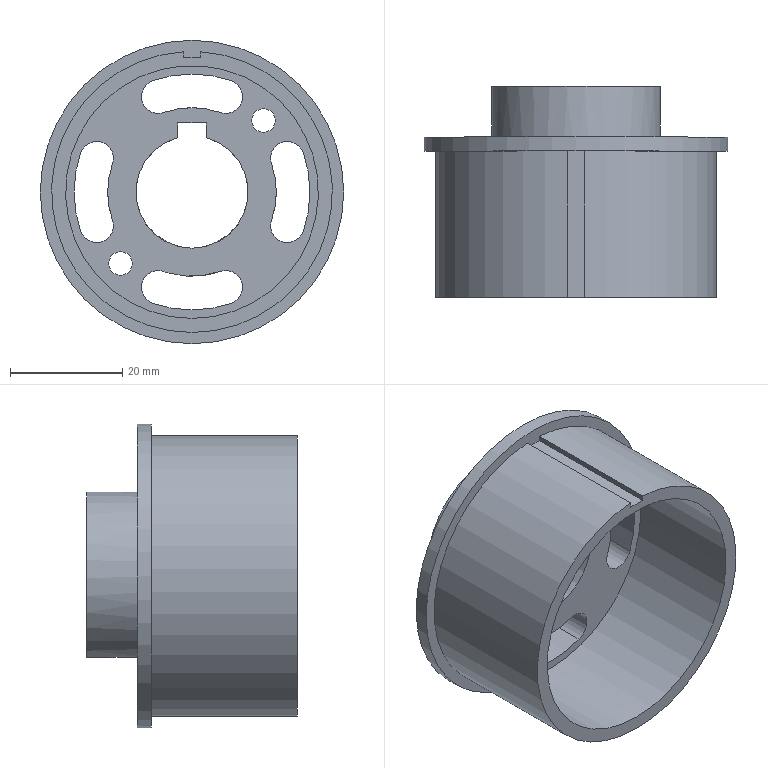Part | NX | features BREP 1 | 1 solid | 33 faces | box 54 x 37.5 x 54 mm | volume 20240 mm3 | cylinder 19 | plane 14 | commonest cylinder face diameters 6 x8 42 x4 4.2 x2 20 x1 30 x1 45 x1
STEP:
#1=CARTESIAN_POINT('',(2648.223,4020.914,39.054));
#2=VERTEX_POINT('',#1);
#3=CARTESIAN_POINT('',(2648.223,4020.914,36.954));
#4=DIRECTION('',(0.,1.,0.));
#5=DIRECTION('',(0.,0.,1.));
#6=AXIS2_PLACEMENT_3D('',#3,#4,#5);
#7=CIRCLE('',#6,2.1);
#8=EDGE_CURVE('',#2,#2,#7,.T.);
#9=ORIENTED_EDGE('',*,*,#8,.T.);
#10=EDGE_LOOP('',(#9));
#11=FACE_BOUND('',#10,.T.);
#12=CARTESIAN_POINT('',(2648.223,4013.914,39.054));
#13=VERTEX_POINT('',#12);
#14=CARTESIAN_POINT('',(2648.223,4013.914,36.954));
#15=DIRECTION('',(0.,1.,0.));
#16=DIRECTION('',(0.,0.,1.));
#17=AXIS2_PLACEMENT_3D('',#14,#15,#16);
#18=CIRCLE('',#17,2.1);
#19=EDGE_CURVE('',#13,#13,#18,.T.);
#20=ORIENTED_EDGE('',*,*,#19,.F.);
#21=EDGE_LOOP('',(#20));
#22=FACE_BOUND('',#21,.T.);
#23=CARTESIAN_POINT('',(2648.223,4020.914,36.954));
#24=DIRECTION('',(0.,1.,0.));
#25=DIRECTION('',(0.,0.,1.));
#26=AXIS2_PLACEMENT_3D('',#23,#24,#25);
#27=CYLINDRICAL_SURFACE('',#26,2.1);
#28=ADVANCED_FACE('',(#11,#22),#27,.F.);
#29=CARTESIAN_POINT('',(2673.679,4020.914,64.51));
#30=VERTEX_POINT('',#29);
#31=CARTESIAN_POINT('',(2673.679,4020.914,62.41));
#32=DIRECTION('',(0.,1.,0.));
#33=DIRECTION('',(0.,0.,1.));
#34=AXIS2_PLACEMENT_3D('',#31,#32,#33);
#35=CIRCLE('',#34,2.1);
#36=EDGE_CURVE('',#30,#30,#35,.T.);
#37=ORIENTED_EDGE('',*,*,#36,.T.);
#38=EDGE_LOOP('',(#37));
#39=FACE_BOUND('',#38,.T.);
#40=CARTESIAN_POINT('',(2673.679,4013.914,64.51));
#41=VERTEX_POINT('',#40);
#42=CARTESIAN_POINT('',(2673.679,4013.914,62.41));
#43=DIRECTION('',(0.,1.,0.));
#44=DIRECTION('',(0.,0.,1.));
#45=AXIS2_PLACEMENT_3D('',#42,#43,#44);
#46=CIRCLE('',#45,2.1);
#47=EDGE_CURVE('',#41,#41,#46,.T.);
#48=ORIENTED_EDGE('',*,*,#47,.F.);
#49=EDGE_LOOP('',(#48));
#50=FACE_BOUND('',#49,.T.);
#51=CARTESIAN_POINT('',(2673.679,4020.914,62.41));
#52=DIRECTION('',(0.,1.,0.));
#53=DIRECTION('',(0.,0.,1.));
#54=AXIS2_PLACEMENT_3D('',#51,#52,#53);
#55=CYLINDRICAL_SURFACE('',#54,2.1);
#56=ADVANCED_FACE('',(#39,#50),#55,.F.);
#57=CARTESIAN_POINT('',(2641.152,4013.914,56.682));
#58=VERTEX_POINT('',#57);
#59=CARTESIAN_POINT('',(2646.809,4013.914,54.682));
#60=VERTEX_POINT('',#59);
#61=CARTESIAN_POINT('',(2643.98,4013.914,55.682));
#62=DIRECTION('',(0.,1.,0.));
#63=DIRECTION('',(0.,0.,1.));
#64=AXIS2_PLACEMENT_3D('',#61,#62,#63);
#65=CIRCLE('',#64,3.);
#66=EDGE_CURVE('',#58,#60,#65,.T.);
#67=ORIENTED_EDGE('',*,*,#66,.F.);
#68=CARTESIAN_POINT('',(2641.152,4020.914,56.682));
#69=VERTEX_POINT('',#68);
#70=CARTESIAN_POINT('',(2641.152,4010.914,56.682));
#71=DIRECTION('',(0.,1.,0.));
#72=VECTOR('',#71,1000.);
#73=LINE('',#70,#72);
#74=EDGE_CURVE('',#58,#69,#73,.T.);
#75=ORIENTED_EDGE('',*,*,#74,.T.);
#76=CARTESIAN_POINT('',(2646.809,4020.914,54.682));
#77=VERTEX_POINT('',#76);
#78=CARTESIAN_POINT('',(2643.98,4020.914,55.682));
#79=DIRECTION('',(0.,1.,0.));
#80=DIRECTION('',(1.,0.,0.));
#81=AXIS2_PLACEMENT_3D('',#78,#79,#80);
#82=CIRCLE('',#81,3.);
#83=EDGE_CURVE('',#69,#77,#82,.T.);
#84=ORIENTED_EDGE('',*,*,#83,.T.);
#85=CARTESIAN_POINT('',(2646.809,4010.914,54.682));
#86=DIRECTION('',(0.,1.,0.));
#87=VECTOR('',#86,1000.);
#88=LINE('',#85,#87);
#89=EDGE_CURVE('',#60,#77,#88,.T.);
#90=ORIENTED_EDGE('',*,*,#89,.F.);
#91=EDGE_LOOP('',(#67,#75,#84,#90));
#92=FACE_BOUND('',#91,.T.);
#93=CARTESIAN_POINT('',(2643.98,4010.914,55.682));
#94=DIRECTION('',(0.,1.,0.));
#95=DIRECTION('',(0.,0.,1.));
#96=AXIS2_PLACEMENT_3D('',#93,#94,#95);
#97=CYLINDRICAL_SURFACE('',#96,3.);
#98=ADVANCED_FACE('',(#92),#97,.F.);
#99=CARTESIAN_POINT('',(2653.951,4013.914,69.481));
#100=VERTEX_POINT('',#99);
#101=CARTESIAN_POINT('',(2667.951,4013.914,69.481));
#102=VERTEX_POINT('',#101);
#103=CARTESIAN_POINT('',(2660.951,4013.914,49.682));
#104=DIRECTION('',(0.,1.,0.));
#105=DIRECTION('',(0.,0.,1.));
#106=AXIS2_PLACEMENT_3D('',#103,#104,#105);
#107=CIRCLE('',#106,21.);
#108=EDGE_CURVE('',#100,#102,#107,.T.);
#109=ORIENTED_EDGE('',*,*,#108,.F.);
#110=CARTESIAN_POINT('',(2653.951,4020.914,69.481));
#111=VERTEX_POINT('',#110);
#112=CARTESIAN_POINT('',(2653.951,4010.914,69.481));
#113=DIRECTION('',(0.,1.,0.));
#114=VECTOR('',#113,1000.);
#115=LINE('',#112,#114);
#116=EDGE_CURVE('',#100,#111,#115,.T.);
#117=ORIENTED_EDGE('',*,*,#116,.T.);
#118=CARTESIAN_POINT('',(2667.951,4020.914,69.481));
#119=VERTEX_POINT('',#118);
#120=CARTESIAN_POINT('',(2660.951,4020.914,49.682));
#121=DIRECTION('',(0.,1.,0.));
#122=DIRECTION('',(0.,0.,-1.));
#123=AXIS2_PLACEMENT_3D('',#120,#121,#122);
#124=CIRCLE('',#123,21.);
#125=EDGE_CURVE('',#111,#119,#124,.T.);
#126=ORIENTED_EDGE('',*,*,#125,.T.);
#127=CARTESIAN_POINT('',(2667.951,4010.914,69.481));
#128=DIRECTION('',(0.,1.,0.));
#129=VECTOR('',#128,1000.);
#130=LINE('',#127,#129);
#131=EDGE_CURVE('',#102,#119,#130,.T.);
#132=ORIENTED_EDGE('',*,*,#131,.F.);
#133=EDGE_LOOP('',(#109,#117,#126,#132));
#134=FACE_BOUND('',#133,.T.);
#135=CARTESIAN_POINT('',(2660.951,4010.914,49.682));
#136=DIRECTION('',(0.,1.,0.));
#137=DIRECTION('',(0.,0.,1.));
#138=AXIS2_PLACEMENT_3D('',#135,#136,#137);
#139=CYLINDRICAL_SURFACE('',#138,21.);
#140=ADVANCED_FACE('',(#134),#139,.F.);
#141=CARTESIAN_POINT('',(2675.093,4013.914,54.682));
#142=VERTEX_POINT('',#141);
#143=CARTESIAN_POINT('',(2680.75,4013.914,56.682));
#144=VERTEX_POINT('',#143);
#145=CARTESIAN_POINT('',(2677.922,4013.914,55.682));
#146=DIRECTION('',(0.,1.,0.));
#147=DIRECTION('',(0.,0.,1.));
#148=AXIS2_PLACEMENT_3D('',#145,#146,#147);
#149=CIRCLE('',#148,3.);
#150=EDGE_CURVE('',#142,#144,#149,.T.);
#151=ORIENTED_EDGE('',*,*,#150,.F.);
#152=CARTESIAN_POINT('',(2675.093,4020.914,54.682));
#153=VERTEX_POINT('',#152);
#154=CARTESIAN_POINT('',(2675.093,4010.914,54.682));
#155=DIRECTION('',(0.,1.,0.));
#156=VECTOR('',#155,1000.);
#157=LINE('',#154,#156);
#158=EDGE_CURVE('',#142,#153,#157,.T.);
#159=ORIENTED_EDGE('',*,*,#158,.T.);
#160=CARTESIAN_POINT('',(2680.75,4020.914,56.682));
#161=VERTEX_POINT('',#160);
#162=CARTESIAN_POINT('',(2677.922,4020.914,55.682));
#163=DIRECTION('',(0.,1.,0.));
#164=DIRECTION('',(-1.,0.,0.));
#165=AXIS2_PLACEMENT_3D('',#162,#163,#164);
#166=CIRCLE('',#165,3.);
#167=EDGE_CURVE('',#153,#161,#166,.T.);
#168=ORIENTED_EDGE('',*,*,#167,.T.);
#169=CARTESIAN_POINT('',(2680.75,4010.914,56.682));
#170=DIRECTION('',(0.,1.,0.));
#171=VECTOR('',#170,1000.);
#172=LINE('',#169,#171);
#173=EDGE_CURVE('',#144,#161,#172,.T.);
#174=ORIENTED_EDGE('',*,*,#173,.F.);
#175=EDGE_LOOP('',(#151,#159,#168,#174));
#176=FACE_BOUND('',#175,.T.);
#177=CARTESIAN_POINT('',(2677.922,4010.914,55.682));
#178=DIRECTION('',(0.,1.,0.));
#179=DIRECTION('',(0.,0.,1.));
#180=AXIS2_PLACEMENT_3D('',#177,#178,#179);
#181=CYLINDRICAL_SURFACE('',#180,3.);
#182=ADVANCED_FACE('',(#176),#181,.F.);
#183=CARTESIAN_POINT('',(2653.951,4013.914,29.883));
#184=VERTEX_POINT('',#183);
#185=CARTESIAN_POINT('',(2655.951,4013.914,35.54));
#186=VERTEX_POINT('',#185);
#187=CARTESIAN_POINT('',(2654.951,4013.914,32.712));
#188=DIRECTION('',(0.,1.,0.));
#189=DIRECTION('',(0.,0.,1.));
#190=AXIS2_PLACEMENT_3D('',#187,#188,#189);
#191=CIRCLE('',#190,3.);
#192=EDGE_CURVE('',#184,#186,#191,.T.);
#193=ORIENTED_EDGE('',*,*,#192,.F.);
#194=CARTESIAN_POINT('',(2653.951,4020.914,29.883));
#195=VERTEX_POINT('',#194);
#196=CARTESIAN_POINT('',(2653.951,4010.914,29.883));
#197=DIRECTION('',(0.,1.,0.));
#198=VECTOR('',#197,1000.);
#199=LINE('',#196,#198);
#200=EDGE_CURVE('',#184,#195,#199,.T.);
#201=ORIENTED_EDGE('',*,*,#200,.T.);
#202=CARTESIAN_POINT('',(2655.951,4020.914,35.54));
#203=VERTEX_POINT('',#202);
#204=CARTESIAN_POINT('',(2654.951,4020.914,32.712));
#205=DIRECTION('',(0.,1.,0.));
#206=DIRECTION('',(0.,0.,1.));
#207=AXIS2_PLACEMENT_3D('',#204,#205,#206);
#208=CIRCLE('',#207,3.);
#209=EDGE_CURVE('',#195,#203,#208,.T.);
#210=ORIENTED_EDGE('',*,*,#209,.T.);
#211=CARTESIAN_POINT('',(2655.951,4010.914,35.54));
#212=DIRECTION('',(0.,1.,0.));
#213=VECTOR('',#212,1000.);
#214=LINE('',#211,#213);
#215=EDGE_CURVE('',#186,#203,#214,.T.);
#216=ORIENTED_EDGE('',*,*,#215,.F.);
#217=EDGE_LOOP('',(#193,#201,#210,#216));
#218=FACE_BOUND('',#217,.T.);
#219=CARTESIAN_POINT('',(2654.951,4010.914,32.712));
#220=DIRECTION('',(0.,1.,0.));
#221=DIRECTION('',(0.,0.,1.));
#222=AXIS2_PLACEMENT_3D('',#219,#220,#221);
#223=CYLINDRICAL_SURFACE('',#222,3.);
#224=ADVANCED_FACE('',(#218),#223,.F.);
#225=CARTESIAN_POINT('',(2665.951,4013.914,35.54));
#226=VERTEX_POINT('',#225);
#227=CARTESIAN_POINT('',(2667.951,4013.914,29.883));
#228=VERTEX_POINT('',#227);
#229=CARTESIAN_POINT('',(2666.951,4013.914,32.712));
#230=DIRECTION('',(0.,1.,0.));
#231=DIRECTION('',(0.,0.,1.));
#232=AXIS2_PLACEMENT_3D('',#229,#230,#231);
#233=CIRCLE('',#232,3.);
#234=EDGE_CURVE('',#226,#228,#233,.T.);
#235=ORIENTED_EDGE('',*,*,#234,.F.);
#236=CARTESIAN_POINT('',(2665.951,4020.914,35.54));
#237=VERTEX_POINT('',#236);
#238=CARTESIAN_POINT('',(2665.951,4010.914,35.54));
#239=DIRECTION('',(0.,1.,0.));
#240=VECTOR('',#239,1000.);
#241=LINE('',#238,#240);
#242=EDGE_CURVE('',#226,#237,#241,.T.);
#243=ORIENTED_EDGE('',*,*,#242,.T.);
#244=CARTESIAN_POINT('',(2667.951,4020.914,29.883));
#245=VERTEX_POINT('',#244);
#246=CARTESIAN_POINT('',(2666.951,4020.914,32.712));
#247=DIRECTION('',(0.,1.,0.));
#248=DIRECTION('',(0.,0.,1.));
#249=AXIS2_PLACEMENT_3D('',#246,#247,#248);
#250=CIRCLE('',#249,3.);
#251=EDGE_CURVE('',#237,#245,#250,.T.);
#252=ORIENTED_EDGE('',*,*,#251,.T.);
#253=CARTESIAN_POINT('',(2667.951,4010.914,29.883));
#254=DIRECTION('',(0.,1.,0.));
#255=VECTOR('',#254,1000.);
#256=LINE('',#253,#255);
#257=EDGE_CURVE('',#228,#245,#256,.T.);
#258=ORIENTED_EDGE('',*,*,#257,.F.);
#259=EDGE_LOOP('',(#235,#243,#252,#258));
#260=FACE_BOUND('',#259,.T.);
#261=CARTESIAN_POINT('',(2666.951,4010.914,32.712));
#262=DIRECTION('',(0.,1.,0.));
#263=DIRECTION('',(0.,0.,1.));
#264=AXIS2_PLACEMENT_3D('',#261,#262,#263);
#265=CYLINDRICAL_SURFACE('',#264,3.);
#266=ADVANCED_FACE('',(#260),#265,.F.);
#267=CARTESIAN_POINT('',(2660.951,3992.414,27.182));
#268=VERTEX_POINT('',#267);
#269=CARTESIAN_POINT('',(2660.951,3992.414,49.682));
#270=DIRECTION('',(0.,-1.,0.));
#271=DIRECTION('',(0.,0.,-1.));
#272=AXIS2_PLACEMENT_3D('',#269,#270,#271);
#273=CIRCLE('',#272,22.5);
#274=EDGE_CURVE('',#268,#268,#273,.T.);
#275=ORIENTED_EDGE('',*,*,#274,.T.);
#276=EDGE_LOOP('',(#275));
#277=FACE_BOUND('',#276,.T.);
#278=CARTESIAN_POINT('',(2660.951,4013.914,27.182));
#279=VERTEX_POINT('',#278);
#280=CARTESIAN_POINT('',(2660.951,4013.914,49.682));
#281=DIRECTION('',(0.,-1.,0.));
#282=DIRECTION('',(0.,0.,-1.));
#283=AXIS2_PLACEMENT_3D('',#280,#281,#282);
#284=CIRCLE('',#283,22.5);
#285=EDGE_CURVE('',#279,#279,#284,.T.);
#286=ORIENTED_EDGE('',*,*,#285,.F.);
#287=EDGE_LOOP('',(#286));
#288=FACE_BOUND('',#287,.T.);
#289=CARTESIAN_POINT('',(2660.951,4029.914,49.682));
#290=DIRECTION('',(0.,-1.,0.));
#291=DIRECTION('',(0.,0.,-1.));
#292=AXIS2_PLACEMENT_3D('',#289,#290,#291);
#293=CYLINDRICAL_SURFACE('',#292,22.5);
#294=ADVANCED_FACE('',(#277,#288),#293,.F.);
#295=CARTESIAN_POINT('',(2660.951,4013.914,49.682));
#296=DIRECTION('',(0.,-1.,0.));
#297=DIRECTION('',(0.,0.,1.));
#298=AXIS2_PLACEMENT_3D('',#295,#296,#297);
#299=CIRCLE('',#298,15.);
#300=EDGE_CURVE('',#186,#226,#299,.T.);
#301=ORIENTED_EDGE('',*,*,#300,.F.);
#302=ORIENTED_EDGE('',*,*,#215,.T.);
#303=CARTESIAN_POINT('',(2646.809,4020.914,44.682));
#304=VERTEX_POINT('',#303);
#305=CARTESIAN_POINT('',(2660.951,4020.914,49.682));
#306=DIRECTION('',(0.,1.,0.));
#307=DIRECTION('',(0.,0.,1.));
#308=AXIS2_PLACEMENT_3D('',#305,#306,#307);
#309=CIRCLE('',#308,15.);
#310=EDGE_CURVE('',#203,#304,#309,.T.);
#311=ORIENTED_EDGE('',*,*,#310,.T.);
#312=CARTESIAN_POINT('',(2646.809,4013.914,44.682));
#313=VERTEX_POINT('',#312);
#314=CARTESIAN_POINT('',(2646.809,4010.914,44.682));
#315=DIRECTION('',(0.,1.,0.));
#316=VECTOR('',#315,1000.);
#317=LINE('',#314,#316);
#318=EDGE_CURVE('',#313,#304,#317,.T.);
#319=ORIENTED_EDGE('',*,*,#318,.F.);
#320=CARTESIAN_POINT('',(2660.951,4013.914,49.682));
#321=DIRECTION('',(0.,-1.,0.));
#322=DIRECTION('',(0.,0.,1.));
#323=AXIS2_PLACEMENT_3D('',#320,#321,#322);
#324=CIRCLE('',#323,15.);
#325=EDGE_CURVE('',#60,#313,#324,.T.);
#326=ORIENTED_EDGE('',*,*,#325,.F.);
#327=ORIENTED_EDGE('',*,*,#89,.T.);
#328=CARTESIAN_POINT('',(2655.951,4020.914,63.825));
#329=VERTEX_POINT('',#328);
#330=CARTESIAN_POINT('',(2660.951,4020.914,49.682));
#331=DIRECTION('',(0.,1.,0.));
#332=DIRECTION('',(0.,0.,1.));
#333=AXIS2_PLACEMENT_3D('',#330,#331,#332);
#334=CIRCLE('',#333,15.);
#335=EDGE_CURVE('',#77,#329,#334,.T.);
#336=ORIENTED_EDGE('',*,*,#335,.T.);
#337=CARTESIAN_POINT('',(2655.951,4013.914,63.825));
#338=VERTEX_POINT('',#337);
#339=CARTESIAN_POINT('',(2655.951,4010.914,63.825));
#340=DIRECTION('',(0.,1.,0.));
#341=VECTOR('',#340,1000.);
#342=LINE('',#339,#341);
#343=EDGE_CURVE('',#338,#329,#342,.T.);
#344=ORIENTED_EDGE('',*,*,#343,.F.);
#345=CARTESIAN_POINT('',(2665.951,4013.914,63.825));
#346=VERTEX_POINT('',#345);
#347=CARTESIAN_POINT('',(2660.951,4013.914,49.682));
#348=DIRECTION('',(0.,-1.,0.));
#349=DIRECTION('',(0.,0.,1.));
#350=AXIS2_PLACEMENT_3D('',#347,#348,#349);
#351=CIRCLE('',#350,15.);
#352=EDGE_CURVE('',#346,#338,#351,.T.);
#353=ORIENTED_EDGE('',*,*,#352,.F.);
#354=CARTESIAN_POINT('',(2665.951,4020.914,63.825));
#355=VERTEX_POINT('',#354);
#356=CARTESIAN_POINT('',(2665.951,4010.914,63.825));
#357=DIRECTION('',(0.,1.,0.));
#358=VECTOR('',#357,1000.);
#359=LINE('',#356,#358);
#360=EDGE_CURVE('',#346,#355,#359,.T.);
#361=ORIENTED_EDGE('',*,*,#360,.T.);
#362=CARTESIAN_POINT('',(2660.951,4020.914,49.682));
#363=DIRECTION('',(0.,1.,0.));
#364=DIRECTION('',(0.,0.,1.));
#365=AXIS2_PLACEMENT_3D('',#362,#363,#364);
#366=CIRCLE('',#365,15.);
#367=EDGE_CURVE('',#355,#153,#366,.T.);
#368=ORIENTED_EDGE('',*,*,#367,.T.);
#369=ORIENTED_EDGE('',*,*,#158,.F.);
#370=CARTESIAN_POINT('',(2675.093,4013.914,44.682));
#371=VERTEX_POINT('',#370);
#372=CARTESIAN_POINT('',(2660.951,4013.914,49.682));
#373=DIRECTION('',(0.,-1.,0.));
#374=DIRECTION('',(0.,0.,1.));
#375=AXIS2_PLACEMENT_3D('',#372,#373,#374);
#376=CIRCLE('',#375,15.);
#377=EDGE_CURVE('',#371,#142,#376,.T.);
#378=ORIENTED_EDGE('',*,*,#377,.F.);
#379=CARTESIAN_POINT('',(2675.093,4020.914,44.682));
#380=VERTEX_POINT('',#379);
#381=CARTESIAN_POINT('',(2675.093,4010.914,44.682));
#382=DIRECTION('',(0.,1.,0.));
#383=VECTOR('',#382,1000.);
#384=LINE('',#381,#383);
#385=EDGE_CURVE('',#371,#380,#384,.T.);
#386=ORIENTED_EDGE('',*,*,#385,.T.);
#387=CARTESIAN_POINT('',(2660.951,4020.914,49.682));
#388=DIRECTION('',(0.,1.,0.));
#389=DIRECTION('',(0.,0.,1.));
#390=AXIS2_PLACEMENT_3D('',#387,#388,#389);
#391=CIRCLE('',#390,15.);
#392=EDGE_CURVE('',#380,#237,#391,.T.);
#393=ORIENTED_EDGE('',*,*,#392,.T.);
#394=ORIENTED_EDGE('',*,*,#242,.F.);
#395=EDGE_LOOP('',(#301,#302,#311,#319,#326,#327,#336,#344,#353,#361,#368,#369,#378,#386,#393,#394));
#396=FACE_BOUND('',#395,.T.);
#397=CARTESIAN_POINT('',(2656.951,4029.914,35.226));
#398=VERTEX_POINT('',#397);
#399=CARTESIAN_POINT('',(2664.951,4029.914,35.226));
#400=VERTEX_POINT('',#399);
#401=CARTESIAN_POINT('',(2660.951,4029.914,49.682));
#402=DIRECTION('',(0.,1.,0.));
#403=DIRECTION('',(0.,0.,1.));
#404=AXIS2_PLACEMENT_3D('',#401,#402,#403);
#405=CIRCLE('',#404,15.);
#406=EDGE_CURVE('',#398,#400,#405,.T.);
#407=ORIENTED_EDGE('',*,*,#406,.F.);
#408=CARTESIAN_POINT('',(2656.951,4020.914,35.226));
#409=VERTEX_POINT('',#408);
#410=CARTESIAN_POINT('',(2656.951,4020.914,35.226));
#411=DIRECTION('',(0.,1.,0.));
#412=VECTOR('',#411,1000.);
#413=LINE('',#410,#412);
#414=EDGE_CURVE('',#409,#398,#413,.T.);
#415=ORIENTED_EDGE('',*,*,#414,.F.);
#416=CARTESIAN_POINT('',(2664.951,4020.914,35.226));
#417=VERTEX_POINT('',#416);
#418=CARTESIAN_POINT('',(2660.951,4020.914,49.682));
#419=DIRECTION('',(0.,-1.,0.));
#420=DIRECTION('',(0.,0.,1.));
#421=AXIS2_PLACEMENT_3D('',#418,#419,#420);
#422=CIRCLE('',#421,15.);
#423=EDGE_CURVE('',#409,#417,#422,.T.);
#424=ORIENTED_EDGE('',*,*,#423,.T.);
#425=CARTESIAN_POINT('',(2664.951,4020.914,35.226));
#426=DIRECTION('',(0.,1.,0.));
#427=VECTOR('',#426,1000.);
#428=LINE('',#425,#427);
#429=EDGE_CURVE('',#417,#400,#428,.T.);
#430=ORIENTED_EDGE('',*,*,#429,.T.);
#431=EDGE_LOOP('',(#407,#415,#424,#430));
#432=FACE_BOUND('',#431,.T.);
#433=CARTESIAN_POINT('',(2660.951,4029.914,49.682));
#434=DIRECTION('',(0.,-1.,0.));
#435=DIRECTION('',(0.,0.,-1.));
#436=AXIS2_PLACEMENT_3D('',#433,#434,#435);
#437=CYLINDRICAL_SURFACE('',#436,15.);
#438=ADVANCED_FACE('',(#396,#432),#437,.T.);
#439=CARTESIAN_POINT('',(2660.951,4018.414,22.682));
#440=VERTEX_POINT('',#439);
#441=CARTESIAN_POINT('',(2660.951,4018.414,49.682));
#442=DIRECTION('',(0.,-1.,0.));
#443=DIRECTION('',(0.,0.,-1.));
#444=AXIS2_PLACEMENT_3D('',#441,#442,#443);
#445=CIRCLE('',#444,27.);
#446=EDGE_CURVE('',#440,#440,#445,.T.);
#447=ORIENTED_EDGE('',*,*,#446,.F.);
#448=EDGE_LOOP('',(#447));
#449=FACE_BOUND('',#448,.T.);
#450=CARTESIAN_POINT('',(2660.951,4020.914,22.682));
#451=VERTEX_POINT('',#450);
#452=CARTESIAN_POINT('',(2660.951,4020.914,49.682));
#453=DIRECTION('',(0.,-1.,0.));
#454=DIRECTION('',(0.,0.,-1.));
#455=AXIS2_PLACEMENT_3D('',#452,#453,#454);
#456=CIRCLE('',#455,27.);
#457=EDGE_CURVE('',#451,#451,#456,.T.);
#458=ORIENTED_EDGE('',*,*,#457,.T.);
#459=EDGE_LOOP('',(#458));
#460=FACE_BOUND('',#459,.T.);
#461=CARTESIAN_POINT('',(2660.951,4020.914,49.682));
#462=DIRECTION('',(0.,-1.,0.));
#463=DIRECTION('',(0.,0.,-1.));
#464=AXIS2_PLACEMENT_3D('',#461,#462,#463);
#465=CYLINDRICAL_SURFACE('',#464,27.);
#466=ADVANCED_FACE('',(#449,#460),#465,.T.);
#467=CARTESIAN_POINT('',(2656.951,4020.914,40.517));
#468=VERTEX_POINT('',#467);
#469=CARTESIAN_POINT('',(2664.951,4020.914,40.517));
#470=VERTEX_POINT('',#469);
#471=CARTESIAN_POINT('',(2660.951,4020.914,49.682));
#472=DIRECTION('',(0.,-1.,0.));
#473=DIRECTION('',(0.,0.,-1.));
#474=AXIS2_PLACEMENT_3D('',#471,#472,#473);
#475=CIRCLE('',#474,10.);
#476=EDGE_CURVE('',#468,#470,#475,.T.);
#477=ORIENTED_EDGE('',*,*,#476,.F.);
#478=CARTESIAN_POINT('',(2656.951,4029.914,40.517));
#479=VERTEX_POINT('',#478);
#480=CARTESIAN_POINT('',(2656.951,4020.914,40.517));
#481=DIRECTION('',(0.,1.,0.));
#482=VECTOR('',#481,1000.);
#483=LINE('',#480,#482);
#484=EDGE_CURVE('',#468,#479,#483,.T.);
#485=ORIENTED_EDGE('',*,*,#484,.T.);
#486=CARTESIAN_POINT('',(2658.451,4029.914,59.365));
#487=VERTEX_POINT('',#486);
#488=CARTESIAN_POINT('',(2660.951,4029.914,49.682));
#489=DIRECTION('',(0.,-1.,0.));
#490=DIRECTION('',(0.,0.,-1.));
#491=AXIS2_PLACEMENT_3D('',#488,#489,#490);
#492=CIRCLE('',#491,10.);
#493=EDGE_CURVE('',#487,#479,#492,.T.);
#494=ORIENTED_EDGE('',*,*,#493,.F.);
#495=CARTESIAN_POINT('',(2658.451,4013.914,59.365));
#496=VERTEX_POINT('',#495);
#497=CARTESIAN_POINT('',(2658.451,4029.914,59.365));
#498=DIRECTION('',(0.,1.,0.));
#499=VECTOR('',#498,1000.);
#500=LINE('',#497,#499);
#501=EDGE_CURVE('',#496,#487,#500,.T.);
#502=ORIENTED_EDGE('',*,*,#501,.F.);
#503=CARTESIAN_POINT('',(2663.451,4013.914,59.365));
#504=VERTEX_POINT('',#503);
#505=CARTESIAN_POINT('',(2660.951,4013.914,49.682));
#506=DIRECTION('',(0.,-1.,0.));
#507=DIRECTION('',(0.,0.,-1.));
#508=AXIS2_PLACEMENT_3D('',#505,#506,#507);
#509=CIRCLE('',#508,10.);
#510=EDGE_CURVE('',#496,#504,#509,.T.);
#511=ORIENTED_EDGE('',*,*,#510,.T.);
#512=CARTESIAN_POINT('',(2663.451,4029.914,59.365));
#513=VERTEX_POINT('',#512);
#514=CARTESIAN_POINT('',(2663.451,4029.914,59.365));
#515=DIRECTION('',(0.,-1.,0.));
#516=VECTOR('',#515,1000.);
#517=LINE('',#514,#516);
#518=EDGE_CURVE('',#513,#504,#517,.T.);
#519=ORIENTED_EDGE('',*,*,#518,.F.);
#520=CARTESIAN_POINT('',(2664.951,4029.914,40.517));
#521=VERTEX_POINT('',#520);
#522=CARTESIAN_POINT('',(2660.951,4029.914,49.682));
#523=DIRECTION('',(0.,-1.,0.));
#524=DIRECTION('',(0.,0.,-1.));
#525=AXIS2_PLACEMENT_3D('',#522,#523,#524);
#526=CIRCLE('',#525,10.);
#527=EDGE_CURVE('',#521,#513,#526,.T.);
#528=ORIENTED_EDGE('',*,*,#527,.F.);
#529=CARTESIAN_POINT('',(2664.951,4020.914,40.517));
#530=DIRECTION('',(0.,1.,0.));
#531=VECTOR('',#530,1000.);
#532=LINE('',#529,#531);
#533=EDGE_CURVE('',#470,#521,#532,.T.);
#534=ORIENTED_EDGE('',*,*,#533,.F.);
#535=EDGE_LOOP('',(#477,#485,#494,#502,#511,#519,#528,#534));
#536=FACE_BOUND('',#535,.T.);
#537=CARTESIAN_POINT('',(2660.951,4029.914,49.682));
#538=DIRECTION('',(0.,-1.,0.));
#539=DIRECTION('',(0.,0.,-1.));
#540=AXIS2_PLACEMENT_3D('',#537,#538,#539);
#541=CYLINDRICAL_SURFACE('',#540,10.);
#542=ADVANCED_FACE('',(#536),#541,.F.);
#543=ORIENTED_EDGE('',*,*,#423,.F.);
#544=CARTESIAN_POINT('',(2656.951,4020.914,35.226));
#545=DIRECTION('',(0.,0.,1.));
#546=VECTOR('',#545,1000.);
#547=LINE('',#544,#546);
#548=EDGE_CURVE('',#409,#468,#547,.T.);
#549=ORIENTED_EDGE('',*,*,#548,.T.);
#550=ORIENTED_EDGE('',*,*,#476,.T.);
#551=CARTESIAN_POINT('',(2664.951,4020.914,40.517));
#552=DIRECTION('',(0.,0.,-1.));
#553=VECTOR('',#552,1000.);
#554=LINE('',#551,#553);
#555=EDGE_CURVE('',#470,#417,#554,.T.);
#556=ORIENTED_EDGE('',*,*,#555,.T.);
#557=EDGE_LOOP('',(#543,#549,#550,#556));
#558=FACE_BOUND('',#557,.T.);
#559=CARTESIAN_POINT('',(2687.951,4020.914,49.682));
#560=DIRECTION('',(0.,1.,0.));
#561=DIRECTION('',(0.,0.,1.));
#562=AXIS2_PLACEMENT_3D('',#559,#560,#561);
#563=PLANE('',#562);
#564=ADVANCED_FACE('',(#558),#563,.T.);
#565=CARTESIAN_POINT('',(2658.451,4029.914,61.982));
#566=VERTEX_POINT('',#565);
#567=CARTESIAN_POINT('',(2663.451,4029.914,61.982));
#568=VERTEX_POINT('',#567);
#569=CARTESIAN_POINT('',(2663.451,4029.914,61.982));
#570=DIRECTION('',(1.,0.,0.));
#571=VECTOR('',#570,1000.);
#572=LINE('',#569,#571);
#573=EDGE_CURVE('',#566,#568,#572,.T.);
#574=ORIENTED_EDGE('',*,*,#573,.F.);
#575=CARTESIAN_POINT('',(2658.451,4029.914,57.682));
#576=DIRECTION('',(0.,0.,1.));
#577=VECTOR('',#576,1000.);
#578=LINE('',#575,#577);
#579=EDGE_CURVE('',#487,#566,#578,.T.);
#580=ORIENTED_EDGE('',*,*,#579,.F.);
#581=ORIENTED_EDGE('',*,*,#493,.T.);
#582=CARTESIAN_POINT('',(2656.951,4029.914,35.226));
#583=DIRECTION('',(0.,0.,1.));
#584=VECTOR('',#583,1000.);
#585=LINE('',#582,#584);
#586=EDGE_CURVE('',#398,#479,#585,.T.);
#587=ORIENTED_EDGE('',*,*,#586,.F.);
#588=ORIENTED_EDGE('',*,*,#406,.T.);
#589=CARTESIAN_POINT('',(2664.951,4029.914,40.517));
#590=DIRECTION('',(0.,0.,-1.));
#591=VECTOR('',#590,1000.);
#592=LINE('',#589,#591);
#593=EDGE_CURVE('',#521,#400,#592,.T.);
#594=ORIENTED_EDGE('',*,*,#593,.F.);
#595=ORIENTED_EDGE('',*,*,#527,.T.);
#596=CARTESIAN_POINT('',(2663.451,4029.914,57.682));
#597=DIRECTION('',(0.,0.,1.));
#598=VECTOR('',#597,1000.);
#599=LINE('',#596,#598);
#600=EDGE_CURVE('',#513,#568,#599,.T.);
#601=ORIENTED_EDGE('',*,*,#600,.T.);
#602=EDGE_LOOP('',(#574,#580,#581,#587,#588,#594,#595,#601));
#603=FACE_BOUND('',#602,.T.);
#604=CARTESIAN_POINT('',(2660.951,4029.914,49.682));
#605=DIRECTION('',(0.,1.,0.));
#606=DIRECTION('',(0.,0.,1.));
#607=AXIS2_PLACEMENT_3D('',#604,#605,#606);
#608=PLANE('',#607);
#609=ADVANCED_FACE('',(#603),#608,.T.);
#610=ORIENTED_EDGE('',*,*,#19,.T.);
#611=EDGE_LOOP('',(#610));
#612=FACE_BOUND('',#611,.T.);
#613=ORIENTED_EDGE('',*,*,#47,.T.);
#614=EDGE_LOOP('',(#613));
#615=FACE_BOUND('',#614,.T.);
#616=ORIENTED_EDGE('',*,*,#325,.T.);
#617=CARTESIAN_POINT('',(2641.152,4013.914,42.682));
#618=VERTEX_POINT('',#617);
#619=CARTESIAN_POINT('',(2643.98,4013.914,43.682));
#620=DIRECTION('',(0.,1.,0.));
#621=DIRECTION('',(0.,0.,1.));
#622=AXIS2_PLACEMENT_3D('',#619,#620,#621);
#623=CIRCLE('',#622,3.);
#624=EDGE_CURVE('',#313,#618,#623,.T.);
#625=ORIENTED_EDGE('',*,*,#624,.T.);
#626=CARTESIAN_POINT('',(2660.951,4013.914,49.682));
#627=DIRECTION('',(0.,1.,0.));
#628=DIRECTION('',(0.,0.,1.));
#629=AXIS2_PLACEMENT_3D('',#626,#627,#628);
#630=CIRCLE('',#629,21.);
#631=EDGE_CURVE('',#618,#58,#630,.T.);
#632=ORIENTED_EDGE('',*,*,#631,.T.);
#633=ORIENTED_EDGE('',*,*,#66,.T.);
#634=EDGE_LOOP('',(#616,#625,#632,#633));
#635=FACE_BOUND('',#634,.T.);
#636=ORIENTED_EDGE('',*,*,#352,.T.);
#637=CARTESIAN_POINT('',(2654.951,4013.914,66.653));
#638=DIRECTION('',(0.,1.,0.));
#639=DIRECTION('',(0.,0.,1.));
#640=AXIS2_PLACEMENT_3D('',#637,#638,#639);
#641=CIRCLE('',#640,3.);
#642=EDGE_CURVE('',#338,#100,#641,.T.);
#643=ORIENTED_EDGE('',*,*,#642,.T.);
#644=ORIENTED_EDGE('',*,*,#108,.T.);
#645=CARTESIAN_POINT('',(2666.951,4013.914,66.653));
#646=DIRECTION('',(0.,1.,0.));
#647=DIRECTION('',(0.,0.,1.));
#648=AXIS2_PLACEMENT_3D('',#645,#646,#647);
#649=CIRCLE('',#648,3.);
#650=EDGE_CURVE('',#102,#346,#649,.T.);
#651=ORIENTED_EDGE('',*,*,#650,.T.);
#652=EDGE_LOOP('',(#636,#643,#644,#651));
#653=FACE_BOUND('',#652,.T.);
#654=ORIENTED_EDGE('',*,*,#377,.T.);
#655=ORIENTED_EDGE('',*,*,#150,.T.);
#656=CARTESIAN_POINT('',(2680.75,4013.914,42.682));
#657=VERTEX_POINT('',#656);
#658=CARTESIAN_POINT('',(2660.951,4013.914,49.682));
#659=DIRECTION('',(0.,1.,0.));
#660=DIRECTION('',(0.,0.,1.));
#661=AXIS2_PLACEMENT_3D('',#658,#659,#660);
#662=CIRCLE('',#661,21.);
#663=EDGE_CURVE('',#144,#657,#662,.T.);
#664=ORIENTED_EDGE('',*,*,#663,.T.);
#665=CARTESIAN_POINT('',(2677.922,4013.914,43.682));
#666=DIRECTION('',(0.,1.,0.));
#667=DIRECTION('',(0.,0.,1.));
#668=AXIS2_PLACEMENT_3D('',#665,#666,#667);
#669=CIRCLE('',#668,3.);
#670=EDGE_CURVE('',#657,#371,#669,.T.);
#671=ORIENTED_EDGE('',*,*,#670,.T.);
#672=EDGE_LOOP('',(#654,#655,#664,#671));
#673=FACE_BOUND('',#672,.T.);
#674=ORIENTED_EDGE('',*,*,#192,.T.);
#675=ORIENTED_EDGE('',*,*,#300,.T.);
#676=ORIENTED_EDGE('',*,*,#234,.T.);
#677=CARTESIAN_POINT('',(2660.951,4013.914,49.682));
#678=DIRECTION('',(0.,1.,0.));
#679=DIRECTION('',(0.,0.,1.));
#680=AXIS2_PLACEMENT_3D('',#677,#678,#679);
#681=CIRCLE('',#680,21.);
#682=EDGE_CURVE('',#228,#184,#681,.T.);
#683=ORIENTED_EDGE('',*,*,#682,.T.);
#684=EDGE_LOOP('',(#674,#675,#676,#683));
#685=FACE_BOUND('',#684,.T.);
#686=ORIENTED_EDGE('',*,*,#285,.T.);
#687=EDGE_LOOP('',(#686));
#688=FACE_BOUND('',#687,.T.);
#689=CARTESIAN_POINT('',(2658.451,4013.914,61.982));
#690=VERTEX_POINT('',#689);
#691=CARTESIAN_POINT('',(2658.451,4013.914,49.682));
#692=DIRECTION('',(0.,0.,-1.));
#693=VECTOR('',#692,1000.);
#694=LINE('',#691,#693);
#695=EDGE_CURVE('',#690,#496,#694,.T.);
#696=ORIENTED_EDGE('',*,*,#695,.F.);
#697=CARTESIAN_POINT('',(2663.451,4013.914,61.982));
#698=VERTEX_POINT('',#697);
#699=CARTESIAN_POINT('',(2683.451,4013.914,61.982));
#700=DIRECTION('',(-1.,0.,0.));
#701=VECTOR('',#700,1000.);
#702=LINE('',#699,#701);
#703=EDGE_CURVE('',#698,#690,#702,.T.);
#704=ORIENTED_EDGE('',*,*,#703,.F.);
#705=CARTESIAN_POINT('',(2663.451,4013.914,49.682));
#706=DIRECTION('',(0.,0.,1.));
#707=VECTOR('',#706,1000.);
#708=LINE('',#705,#707);
#709=EDGE_CURVE('',#504,#698,#708,.T.);
#710=ORIENTED_EDGE('',*,*,#709,.F.);
#711=ORIENTED_EDGE('',*,*,#510,.F.);
#712=EDGE_LOOP('',(#696,#704,#710,#711));
#713=FACE_BOUND('',#712,.T.);
#714=CARTESIAN_POINT('',(2683.451,4013.914,49.682));
#715=DIRECTION('',(0.,1.,0.));
#716=DIRECTION('',(0.,0.,1.));
#717=AXIS2_PLACEMENT_3D('',#714,#715,#716);
#718=PLANE('',#717);
#719=ADVANCED_FACE('',(#612,#615,#635,#653,#673,#685,#688,#713),#718,.F.);
#720=ORIENTED_EDGE('',*,*,#446,.T.);
#721=EDGE_LOOP('',(#720));
#722=FACE_BOUND('',#721,.T.);
#723=CARTESIAN_POINT('',(2662.451,4018.414,74.637));
#724=VERTEX_POINT('',#723);
#725=CARTESIAN_POINT('',(2662.451,4018.414,73.682));
#726=VERTEX_POINT('',#725);
#727=CARTESIAN_POINT('',(2662.451,4018.414,73.682));
#728=DIRECTION('',(0.,0.,-1.));
#729=VECTOR('',#728,1000.);
#730=LINE('',#727,#729);
#731=EDGE_CURVE('',#724,#726,#730,.T.);
#732=ORIENTED_EDGE('',*,*,#731,.F.);
#733=CARTESIAN_POINT('',(2659.451,4018.414,74.637));
#734=VERTEX_POINT('',#733);
#735=CARTESIAN_POINT('',(2660.951,4018.414,49.682));
#736=DIRECTION('',(0.,-1.,0.));
#737=DIRECTION('',(0.,0.,-1.));
#738=AXIS2_PLACEMENT_3D('',#735,#736,#737);
#739=CIRCLE('',#738,25.);
#740=EDGE_CURVE('',#734,#724,#739,.T.);
#741=ORIENTED_EDGE('',*,*,#740,.F.);
#742=CARTESIAN_POINT('',(2659.451,4018.414,73.682));
#743=VERTEX_POINT('',#742);
#744=CARTESIAN_POINT('',(2659.451,4018.414,74.637));
#745=DIRECTION('',(0.,0.,1.));
#746=VECTOR('',#745,1000.);
#747=LINE('',#744,#746);
#748=EDGE_CURVE('',#743,#734,#747,.T.);
#749=ORIENTED_EDGE('',*,*,#748,.F.);
#750=CARTESIAN_POINT('',(2659.451,4018.414,73.682));
#751=DIRECTION('',(-1.,0.,0.));
#752=VECTOR('',#751,1000.);
#753=LINE('',#750,#752);
#754=EDGE_CURVE('',#726,#743,#753,.T.);
#755=ORIENTED_EDGE('',*,*,#754,.F.);
#756=EDGE_LOOP('',(#732,#741,#749,#755));
#757=FACE_BOUND('',#756,.T.);
#758=CARTESIAN_POINT('',(2660.951,4018.414,49.682));
#759=DIRECTION('',(0.,-1.,0.));
#760=DIRECTION('',(0.,0.,-1.));
#761=AXIS2_PLACEMENT_3D('',#758,#759,#760);
#762=PLANE('',#761);
#763=ADVANCED_FACE('',(#722,#757),#762,.T.);
#764=ORIENTED_EDGE('',*,*,#8,.F.);
#765=EDGE_LOOP('',(#764));
#766=FACE_BOUND('',#765,.T.);
#767=ORIENTED_EDGE('',*,*,#36,.F.);
#768=EDGE_LOOP('',(#767));
#769=FACE_BOUND('',#768,.T.);
#770=CARTESIAN_POINT('',(2641.152,4020.914,42.682));
#771=VERTEX_POINT('',#770);
#772=CARTESIAN_POINT('',(2643.98,4020.914,43.682));
#773=DIRECTION('',(0.,1.,0.));
#774=DIRECTION('',(1.,0.,0.));
#775=AXIS2_PLACEMENT_3D('',#772,#773,#774);
#776=CIRCLE('',#775,3.);
#777=EDGE_CURVE('',#304,#771,#776,.T.);
#778=ORIENTED_EDGE('',*,*,#777,.F.);
#779=ORIENTED_EDGE('',*,*,#310,.F.);
#780=ORIENTED_EDGE('',*,*,#209,.F.);
#781=CARTESIAN_POINT('',(2660.951,4020.914,49.682));
#782=DIRECTION('',(0.,1.,0.));
#783=DIRECTION('',(0.,0.,1.));
#784=AXIS2_PLACEMENT_3D('',#781,#782,#783);
#785=CIRCLE('',#784,21.);
#786=EDGE_CURVE('',#245,#195,#785,.T.);
#787=ORIENTED_EDGE('',*,*,#786,.F.);
#788=ORIENTED_EDGE('',*,*,#251,.F.);
#789=ORIENTED_EDGE('',*,*,#392,.F.);
#790=CARTESIAN_POINT('',(2680.75,4020.914,42.682));
#791=VERTEX_POINT('',#790);
#792=CARTESIAN_POINT('',(2677.922,4020.914,43.682));
#793=DIRECTION('',(0.,1.,0.));
#794=DIRECTION('',(-1.,0.,0.));
#795=AXIS2_PLACEMENT_3D('',#792,#793,#794);
#796=CIRCLE('',#795,3.);
#797=EDGE_CURVE('',#791,#380,#796,.T.);
#798=ORIENTED_EDGE('',*,*,#797,.F.);
#799=CARTESIAN_POINT('',(2660.951,4020.914,49.682));
#800=DIRECTION('',(0.,1.,0.));
#801=DIRECTION('',(-1.,0.,0.));
#802=AXIS2_PLACEMENT_3D('',#799,#800,#801);
#803=CIRCLE('',#802,21.);
#804=EDGE_CURVE('',#161,#791,#803,.T.);
#805=ORIENTED_EDGE('',*,*,#804,.F.);
#806=ORIENTED_EDGE('',*,*,#167,.F.);
#807=ORIENTED_EDGE('',*,*,#367,.F.);
#808=CARTESIAN_POINT('',(2666.951,4020.914,66.653));
#809=DIRECTION('',(0.,1.,0.));
#810=DIRECTION('',(0.,0.,-1.));
#811=AXIS2_PLACEMENT_3D('',#808,#809,#810);
#812=CIRCLE('',#811,3.);
#813=EDGE_CURVE('',#119,#355,#812,.T.);
#814=ORIENTED_EDGE('',*,*,#813,.F.);
#815=ORIENTED_EDGE('',*,*,#125,.F.);
#816=CARTESIAN_POINT('',(2654.951,4020.914,66.653));
#817=DIRECTION('',(0.,1.,0.));
#818=DIRECTION('',(0.,0.,-1.));
#819=AXIS2_PLACEMENT_3D('',#816,#817,#818);
#820=CIRCLE('',#819,3.);
#821=EDGE_CURVE('',#329,#111,#820,.T.);
#822=ORIENTED_EDGE('',*,*,#821,.F.);
#823=ORIENTED_EDGE('',*,*,#335,.F.);
#824=ORIENTED_EDGE('',*,*,#83,.F.);
#825=CARTESIAN_POINT('',(2660.951,4020.914,49.682));
#826=DIRECTION('',(0.,1.,0.));
#827=DIRECTION('',(1.,0.,0.));
#828=AXIS2_PLACEMENT_3D('',#825,#826,#827);
#829=CIRCLE('',#828,21.);
#830=EDGE_CURVE('',#771,#69,#829,.T.);
#831=ORIENTED_EDGE('',*,*,#830,.F.);
#832=EDGE_LOOP('',(#778,#779,#780,#787,#788,#789,#798,#805,#806,#807,#814,#815,#822,#823,#824,#831));
#833=FACE_BOUND('',#832,.T.);
#834=ORIENTED_EDGE('',*,*,#457,.F.);
#835=EDGE_LOOP('',(#834));
#836=FACE_BOUND('',#835,.T.);
#837=CARTESIAN_POINT('',(2687.951,4020.914,49.682));
#838=DIRECTION('',(0.,1.,0.));
#839=DIRECTION('',(0.,0.,1.));
#840=AXIS2_PLACEMENT_3D('',#837,#838,#839);
#841=PLANE('',#840);
#842=ADVANCED_FACE('',(#766,#769,#833,#836),#841,.T.);
#843=ORIENTED_EDGE('',*,*,#593,.T.);
#844=ORIENTED_EDGE('',*,*,#429,.F.);
#845=ORIENTED_EDGE('',*,*,#555,.F.);
#846=ORIENTED_EDGE('',*,*,#533,.T.);
#847=EDGE_LOOP('',(#843,#844,#845,#846));
#848=FACE_BOUND('',#847,.T.);
#849=CARTESIAN_POINT('',(2664.951,4020.914,40.517));
#850=DIRECTION('',(1.,0.,0.));
#851=DIRECTION('',(0.,0.,-1.));
#852=AXIS2_PLACEMENT_3D('',#849,#850,#851);
#853=PLANE('',#852);
#854=ADVANCED_FACE('',(#848),#853,.F.);
#855=ORIENTED_EDGE('',*,*,#586,.T.);
#856=ORIENTED_EDGE('',*,*,#484,.F.);
#857=ORIENTED_EDGE('',*,*,#548,.F.);
#858=ORIENTED_EDGE('',*,*,#414,.T.);
#859=EDGE_LOOP('',(#855,#856,#857,#858));
#860=FACE_BOUND('',#859,.T.);
#861=CARTESIAN_POINT('',(2656.951,4020.914,35.226));
#862=DIRECTION('',(-1.,0.,0.));
#863=DIRECTION('',(0.,0.,1.));
#864=AXIS2_PLACEMENT_3D('',#861,#862,#863);
#865=PLANE('',#864);
#866=ADVANCED_FACE('',(#860),#865,.F.);
#867=ORIENTED_EDGE('',*,*,#740,.T.);
#868=CARTESIAN_POINT('',(2662.451,3992.414,74.637));
#869=VERTEX_POINT('',#868);
#870=CARTESIAN_POINT('',(2662.451,3992.414,74.637));
#871=DIRECTION('',(0.,1.,0.));
#872=VECTOR('',#871,1000.);
#873=LINE('',#870,#872);
#874=EDGE_CURVE('',#869,#724,#873,.T.);
#875=ORIENTED_EDGE('',*,*,#874,.F.);
#876=CARTESIAN_POINT('',(2659.451,3992.414,74.637));
#877=VERTEX_POINT('',#876);
#878=CARTESIAN_POINT('',(2660.951,3992.414,49.682));
#879=DIRECTION('',(0.,-1.,0.));
#880=DIRECTION('',(0.,0.,-1.));
#881=AXIS2_PLACEMENT_3D('',#878,#879,#880);
#882=CIRCLE('',#881,25.);
#883=EDGE_CURVE('',#877,#869,#882,.T.);
#884=ORIENTED_EDGE('',*,*,#883,.F.);
#885=CARTESIAN_POINT('',(2659.451,3992.414,74.637));
#886=DIRECTION('',(0.,1.,0.));
#887=VECTOR('',#886,1000.);
#888=LINE('',#885,#887);
#889=EDGE_CURVE('',#877,#734,#888,.T.);
#890=ORIENTED_EDGE('',*,*,#889,.T.);
#891=EDGE_LOOP('',(#867,#875,#884,#890));
#892=FACE_BOUND('',#891,.T.);
#893=CARTESIAN_POINT('',(2660.951,3992.414,49.682));
#894=DIRECTION('',(0.,1.,0.));
#895=DIRECTION('',(0.,0.,1.));
#896=AXIS2_PLACEMENT_3D('',#893,#894,#895);
#897=CYLINDRICAL_SURFACE('',#896,25.);
#898=ADVANCED_FACE('',(#892),#897,.T.);
#899=ORIENTED_EDGE('',*,*,#731,.T.);
#900=CARTESIAN_POINT('',(2662.451,3992.414,73.682));
#901=VERTEX_POINT('',#900);
#902=CARTESIAN_POINT('',(2662.451,3992.414,73.682));
#903=DIRECTION('',(0.,1.,0.));
#904=VECTOR('',#903,1000.);
#905=LINE('',#902,#904);
#906=EDGE_CURVE('',#901,#726,#905,.T.);
#907=ORIENTED_EDGE('',*,*,#906,.F.);
#908=CARTESIAN_POINT('',(2662.451,3992.414,73.682));
#909=DIRECTION('',(0.,0.,-1.));
#910=VECTOR('',#909,1000.);
#911=LINE('',#908,#910);
#912=EDGE_CURVE('',#869,#901,#911,.T.);
#913=ORIENTED_EDGE('',*,*,#912,.F.);
#914=ORIENTED_EDGE('',*,*,#874,.T.);
#915=EDGE_LOOP('',(#899,#907,#913,#914));
#916=FACE_BOUND('',#915,.T.);
#917=CARTESIAN_POINT('',(2662.451,3992.414,73.682));
#918=DIRECTION('',(1.,0.,0.));
#919=DIRECTION('',(0.,0.,-1.));
#920=AXIS2_PLACEMENT_3D('',#917,#918,#919);
#921=PLANE('',#920);
#922=ADVANCED_FACE('',(#916),#921,.F.);
#923=ORIENTED_EDGE('',*,*,#754,.T.);
#924=CARTESIAN_POINT('',(2659.451,3992.414,73.682));
#925=VERTEX_POINT('',#924);
#926=CARTESIAN_POINT('',(2659.451,3992.414,73.682));
#927=DIRECTION('',(0.,1.,0.));
#928=VECTOR('',#927,1000.);
#929=LINE('',#926,#928);
#930=EDGE_CURVE('',#925,#743,#929,.T.);
#931=ORIENTED_EDGE('',*,*,#930,.F.);
#932=CARTESIAN_POINT('',(2659.451,3992.414,73.682));
#933=DIRECTION('',(-1.,0.,0.));
#934=VECTOR('',#933,1000.);
#935=LINE('',#932,#934);
#936=EDGE_CURVE('',#901,#925,#935,.T.);
#937=ORIENTED_EDGE('',*,*,#936,.F.);
#938=ORIENTED_EDGE('',*,*,#906,.T.);
#939=EDGE_LOOP('',(#923,#931,#937,#938));
#940=FACE_BOUND('',#939,.T.);
#941=CARTESIAN_POINT('',(2659.451,3992.414,73.682));
#942=DIRECTION('',(0.,0.,-1.));
#943=DIRECTION('',(-1.,0.,0.));
#944=AXIS2_PLACEMENT_3D('',#941,#942,#943);
#945=PLANE('',#944);
#946=ADVANCED_FACE('',(#940),#945,.F.);
#947=ORIENTED_EDGE('',*,*,#748,.T.);
#948=ORIENTED_EDGE('',*,*,#889,.F.);
#949=CARTESIAN_POINT('',(2659.451,3992.414,74.637));
#950=DIRECTION('',(0.,0.,1.));
#951=VECTOR('',#950,1000.);
#952=LINE('',#949,#951);
#953=EDGE_CURVE('',#925,#877,#952,.T.);
#954=ORIENTED_EDGE('',*,*,#953,.F.);
#955=ORIENTED_EDGE('',*,*,#930,.T.);
#956=EDGE_LOOP('',(#947,#948,#954,#955));
#957=FACE_BOUND('',#956,.T.);
#958=CARTESIAN_POINT('',(2659.451,3992.414,74.637));
#959=DIRECTION('',(-1.,0.,0.));
#960=DIRECTION('',(0.,0.,1.));
#961=AXIS2_PLACEMENT_3D('',#958,#959,#960);
#962=PLANE('',#961);
#963=ADVANCED_FACE('',(#957),#962,.F.);
#964=ORIENTED_EDGE('',*,*,#274,.F.);
#965=EDGE_LOOP('',(#964));
#966=FACE_BOUND('',#965,.T.);
#967=ORIENTED_EDGE('',*,*,#883,.T.);
#968=ORIENTED_EDGE('',*,*,#912,.T.);
#969=ORIENTED_EDGE('',*,*,#936,.T.);
#970=ORIENTED_EDGE('',*,*,#953,.T.);
#971=EDGE_LOOP('',(#967,#968,#969,#970));
#972=FACE_BOUND('',#971,.T.);
#973=CARTESIAN_POINT('',(2660.951,3992.414,49.682));
#974=DIRECTION('',(0.,-1.,0.));
#975=DIRECTION('',(0.,0.,-1.));
#976=AXIS2_PLACEMENT_3D('',#973,#974,#975);
#977=PLANE('',#976);
#978=ADVANCED_FACE('',(#966,#972),#977,.T.);
#979=ORIENTED_EDGE('',*,*,#501,.T.);
#980=ORIENTED_EDGE('',*,*,#579,.T.);
#981=CARTESIAN_POINT('',(2658.451,4029.914,61.982));
#982=DIRECTION('',(0.,1.,0.));
#983=VECTOR('',#982,1000.);
#984=LINE('',#981,#983);
#985=EDGE_CURVE('',#690,#566,#984,.T.);
#986=ORIENTED_EDGE('',*,*,#985,.F.);
#987=ORIENTED_EDGE('',*,*,#695,.T.);
#988=EDGE_LOOP('',(#979,#980,#986,#987));
#989=FACE_BOUND('',#988,.T.);
#990=CARTESIAN_POINT('',(2658.451,4029.914,57.682));
#991=DIRECTION('',(1.,0.,0.));
#992=DIRECTION('',(0.,0.,-1.));
#993=AXIS2_PLACEMENT_3D('',#990,#991,#992);
#994=PLANE('',#993);
#995=ADVANCED_FACE('',(#989),#994,.T.);
#996=ORIENTED_EDGE('',*,*,#518,.T.);
#997=ORIENTED_EDGE('',*,*,#709,.T.);
#998=CARTESIAN_POINT('',(2663.451,4029.914,61.982));
#999=DIRECTION('',(0.,-1.,0.));
#1000=VECTOR('',#999,1000.);
#1001=LINE('',#998,#1000);
#1002=EDGE_CURVE('',#568,#698,#1001,.T.);
#1003=ORIENTED_EDGE('',*,*,#1002,.F.);
#1004=ORIENTED_EDGE('',*,*,#600,.F.);
#1005=EDGE_LOOP('',(#996,#997,#1003,#1004));
#1006=FACE_BOUND('',#1005,.T.);
#1007=CARTESIAN_POINT('',(2663.451,4029.914,57.682));
#1008=DIRECTION('',(-1.,0.,0.));
#1009=DIRECTION('',(0.,0.,1.));
#1010=AXIS2_PLACEMENT_3D('',#1007,#1008,#1009);
#1011=PLANE('',#1010);
#1012=ADVANCED_FACE('',(#1006),#1011,.T.);
#1013=ORIENTED_EDGE('',*,*,#703,.T.);
#1014=ORIENTED_EDGE('',*,*,#985,.T.);
#1015=ORIENTED_EDGE('',*,*,#573,.T.);
#1016=ORIENTED_EDGE('',*,*,#1002,.T.);
#1017=EDGE_LOOP('',(#1013,#1014,#1015,#1016));
#1018=FACE_BOUND('',#1017,.T.);
#1019=CARTESIAN_POINT('',(0.,0.,61.982));
#1020=DIRECTION('',(0.,0.,-1.));
#1021=DIRECTION('',(-1.,0.,0.));
#1022=AXIS2_PLACEMENT_3D('',#1019,#1020,#1021);
#1023=PLANE('',#1022);
#1024=ADVANCED_FACE('',(#1018),#1023,.T.);
#1025=ORIENTED_EDGE('',*,*,#257,.T.);
#1026=ORIENTED_EDGE('',*,*,#786,.T.);
#1027=ORIENTED_EDGE('',*,*,#200,.F.);
#1028=ORIENTED_EDGE('',*,*,#682,.F.);
#1029=EDGE_LOOP('',(#1025,#1026,#1027,#1028));
#1030=FACE_BOUND('',#1029,.T.);
#1031=CARTESIAN_POINT('',(2660.951,4010.914,49.682));
#1032=DIRECTION('',(0.,1.,0.));
#1033=DIRECTION('',(0.,0.,1.));
#1034=AXIS2_PLACEMENT_3D('',#1031,#1032,#1033);
#1035=CYLINDRICAL_SURFACE('',#1034,21.);
#1036=ADVANCED_FACE('',(#1030),#1035,.F.);
#1037=ORIENTED_EDGE('',*,*,#173,.T.);
#1038=ORIENTED_EDGE('',*,*,#804,.T.);
#1039=CARTESIAN_POINT('',(2680.75,4010.914,42.682));
#1040=DIRECTION('',(0.,1.,0.));
#1041=VECTOR('',#1040,1000.);
#1042=LINE('',#1039,#1041);
#1043=EDGE_CURVE('',#657,#791,#1042,.T.);
#1044=ORIENTED_EDGE('',*,*,#1043,.F.);
#1045=ORIENTED_EDGE('',*,*,#663,.F.);
#1046=EDGE_LOOP('',(#1037,#1038,#1044,#1045));
#1047=FACE_BOUND('',#1046,.T.);
#1048=CARTESIAN_POINT('',(2660.951,4010.914,49.682));
#1049=DIRECTION('',(0.,1.,0.));
#1050=DIRECTION('',(0.,0.,1.));
#1051=AXIS2_PLACEMENT_3D('',#1048,#1049,#1050);
#1052=CYLINDRICAL_SURFACE('',#1051,21.);
#1053=ADVANCED_FACE('',(#1047),#1052,.F.);
#1054=ORIENTED_EDGE('',*,*,#1043,.T.);
#1055=ORIENTED_EDGE('',*,*,#797,.T.);
#1056=ORIENTED_EDGE('',*,*,#385,.F.);
#1057=ORIENTED_EDGE('',*,*,#670,.F.);
#1058=EDGE_LOOP('',(#1054,#1055,#1056,#1057));
#1059=FACE_BOUND('',#1058,.T.);
#1060=CARTESIAN_POINT('',(2677.922,4010.914,43.682));
#1061=DIRECTION('',(0.,1.,0.));
#1062=DIRECTION('',(0.,0.,1.));
#1063=AXIS2_PLACEMENT_3D('',#1060,#1061,#1062);
#1064=CYLINDRICAL_SURFACE('',#1063,3.);
#1065=ADVANCED_FACE('',(#1059),#1064,.F.);
#1066=ORIENTED_EDGE('',*,*,#343,.T.);
#1067=ORIENTED_EDGE('',*,*,#821,.T.);
#1068=ORIENTED_EDGE('',*,*,#116,.F.);
#1069=ORIENTED_EDGE('',*,*,#642,.F.);
#1070=EDGE_LOOP('',(#1066,#1067,#1068,#1069));
#1071=FACE_BOUND('',#1070,.T.);
#1072=CARTESIAN_POINT('',(2654.951,4010.914,66.653));
#1073=DIRECTION('',(0.,1.,0.));
#1074=DIRECTION('',(0.,0.,1.));
#1075=AXIS2_PLACEMENT_3D('',#1072,#1073,#1074);
#1076=CYLINDRICAL_SURFACE('',#1075,3.);
#1077=ADVANCED_FACE('',(#1071),#1076,.F.);
#1078=ORIENTED_EDGE('',*,*,#131,.T.);
#1079=ORIENTED_EDGE('',*,*,#813,.T.);
#1080=ORIENTED_EDGE('',*,*,#360,.F.);
#1081=ORIENTED_EDGE('',*,*,#650,.F.);
#1082=EDGE_LOOP('',(#1078,#1079,#1080,#1081));
#1083=FACE_BOUND('',#1082,.T.);
#1084=CARTESIAN_POINT('',(2666.951,4010.914,66.653));
#1085=DIRECTION('',(0.,1.,0.));
#1086=DIRECTION('',(0.,0.,1.));
#1087=AXIS2_PLACEMENT_3D('',#1084,#1085,#1086);
#1088=CYLINDRICAL_SURFACE('',#1087,3.);
#1089=ADVANCED_FACE('',(#1083),#1088,.F.);
#1090=CARTESIAN_POINT('',(2641.152,4010.914,42.682));
#1091=DIRECTION('',(0.,1.,0.));
#1092=VECTOR('',#1091,1000.);
#1093=LINE('',#1090,#1092);
#1094=EDGE_CURVE('',#618,#771,#1093,.T.);
#1095=ORIENTED_EDGE('',*,*,#1094,.T.);
#1096=ORIENTED_EDGE('',*,*,#830,.T.);
#1097=ORIENTED_EDGE('',*,*,#74,.F.);
#1098=ORIENTED_EDGE('',*,*,#631,.F.);
#1099=EDGE_LOOP('',(#1095,#1096,#1097,#1098));
#1100=FACE_BOUND('',#1099,.T.);
#1101=CARTESIAN_POINT('',(2660.951,4010.914,49.682));
#1102=DIRECTION('',(0.,1.,0.));
#1103=DIRECTION('',(0.,0.,1.));
#1104=AXIS2_PLACEMENT_3D('',#1101,#1102,#1103);
#1105=CYLINDRICAL_SURFACE('',#1104,21.);
#1106=ADVANCED_FACE('',(#1100),#1105,.F.);
#1107=ORIENTED_EDGE('',*,*,#318,.T.);
#1108=ORIENTED_EDGE('',*,*,#777,.T.);
#1109=ORIENTED_EDGE('',*,*,#1094,.F.);
#1110=ORIENTED_EDGE('',*,*,#624,.F.);
#1111=EDGE_LOOP('',(#1107,#1108,#1109,#1110));
#1112=FACE_BOUND('',#1111,.T.);
#1113=CARTESIAN_POINT('',(2643.98,4010.914,43.682));
#1114=DIRECTION('',(0.,1.,0.));
#1115=DIRECTION('',(0.,0.,1.));
#1116=AXIS2_PLACEMENT_3D('',#1113,#1114,#1115);
#1117=CYLINDRICAL_SURFACE('',#1116,3.);
#1118=ADVANCED_FACE('',(#1112),#1117,.F.);
#1119=CLOSED_SHELL('',(#28,#56,#98,#140,#182,#224,#266,#294,#438,#466,#542,#564,#609,#719,#763,#842,#854,#866,#898,#922,#946,#963,#978,#995,#1012,#1024,#1036,#1053,#1065,#1077,#1089,#1106,#1118));
#1120=MANIFOLD_SOLID_BREP('',#1119);
#1121=(LENGTH_UNIT()NAMED_UNIT(*)SI_UNIT(.MILLI.,.METRE.));
#1122=UNCERTAINTY_MEASURE_WITH_UNIT(LENGTH_MEASURE(0.00001),#1121,'','');
#1123=(NAMED_UNIT(*)PLANE_ANGLE_UNIT()SI_UNIT($,.RADIAN.));
#1124=(NAMED_UNIT(*)SI_UNIT($,.STERADIAN.)SOLID_ANGLE_UNIT());
#1125=(GEOMETRIC_REPRESENTATION_CONTEXT(3)GLOBAL_UNCERTAINTY_ASSIGNED_CONTEXT((#1122))GLOBAL_UNIT_ASSIGNED_CONTEXT((#1121,#1123,#1124))REPRESENTATION_CONTEXT('',''));
#1126=ADVANCED_BREP_SHAPE_REPRESENTATION('',(#1120),#1125);